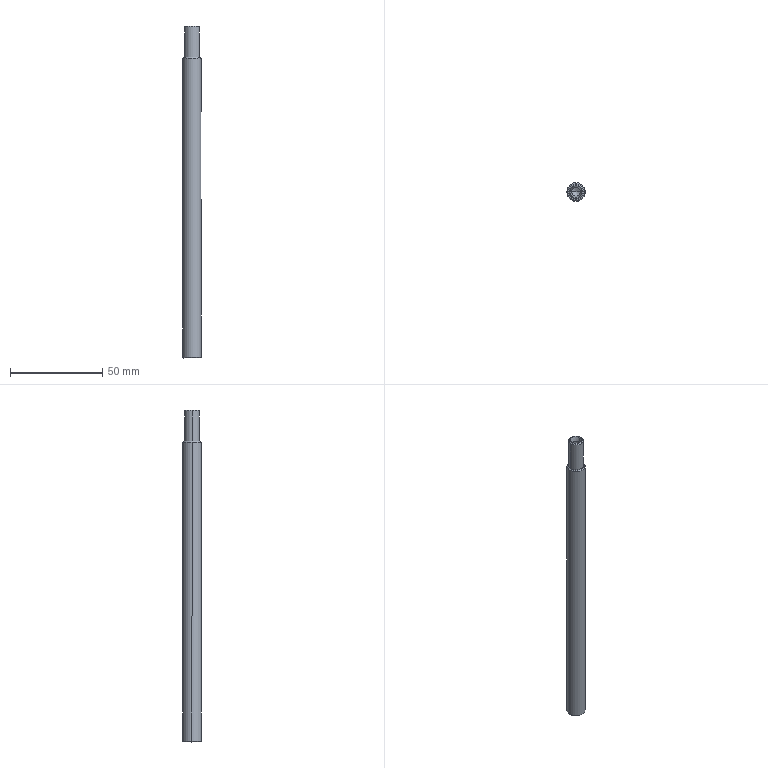Part | SolidWorks | features BaseBody 1 | 1 solid | 30 faces | box 9.9 x 9.9 x 180 mm | volume 12714 mm3 | cone 17 | cylinder 8 | plane 5 | commonest cylinder face diameters 4.8 x2 5 x2 8 x2 9.9 x2